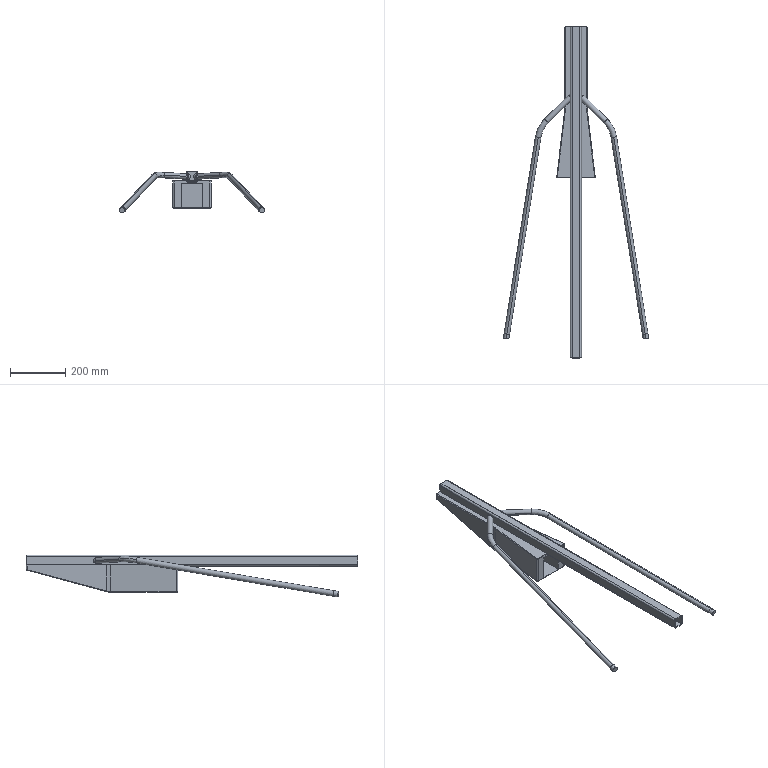Part | SolidWorks | features Fillet 6, ICE 4, 3DProfileFeature 2, MirrorPattern 2, Sweep 1, WeldMemberFeat 1, WeldmentFeature 1 | 1 solid | 114 faces | box 524.94 x 1200 x 151.697 mm | volume 3872299 mm3 | cylinder 52 | plane 31 | spline 19 | torus 12 | commonest cylinder face diameters 20 x21 4 x14 10 x6 6 x4 12 x4 220 x2